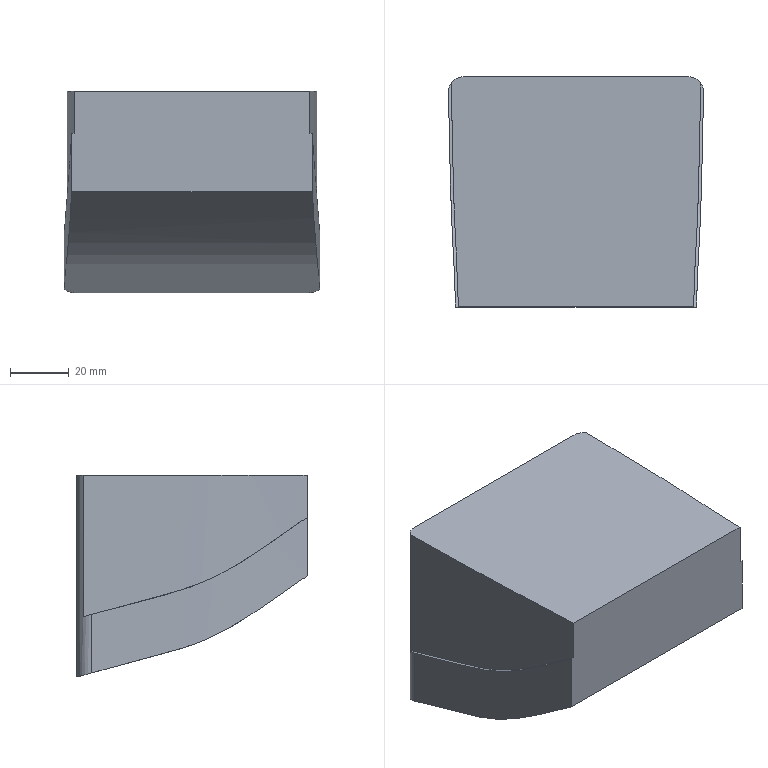Part | NX | features solid 2 | 1 solid | 12 faces | box 87.088 x 78.574 x 68.942 mm | volume 366732 mm3 | spline 7 | plane 3 | cylinder 2 | commonest cylinder face diameters 10 x2
STEP:
#1=CARTESIAN_POINT('',(38.544,100.,30.));
#2=VERTEX_POINT('',#1);
#3=CARTESIAN_POINT('',(-38.544,100.,30.));
#4=VERTEX_POINT('',#3);
#5=CARTESIAN_POINT('',(35.,100.,30.));
#6=DIRECTION('',(1.,0.,0.));
#7=VECTOR('',#6,1000.);
#8=LINE('',#5,#7);
#9=EDGE_CURVE('',#2,#4,#8,.F.);
#10=ORIENTED_EDGE('',*,*,#9,.F.);
#11=CARTESIAN_POINT('',(38.544,100.,-38.942));
#12=VERTEX_POINT('',#11);
#13=CARTESIAN_POINT('',(38.544,100.,-38.942));
#14=DIRECTION('',(0.,0.,1.));
#15=VECTOR('',#14,1000.);
#16=LINE('',#13,#15);
#17=EDGE_CURVE('',#2,#12,#16,.F.);
#18=ORIENTED_EDGE('',*,*,#17,.T.);
#19=CARTESIAN_POINT('',(-38.544,100.,-38.942));
#20=VERTEX_POINT('',#19);
#21=CARTESIAN_POINT('',(0.,100.,-38.942));
#22=DIRECTION('',(1.,0.,0.));
#23=VECTOR('',#22,1000.);
#24=LINE('',#21,#23);
#25=EDGE_CURVE('',#12,#20,#24,.F.);
#26=ORIENTED_EDGE('',*,*,#25,.T.);
#27=CARTESIAN_POINT('',(-38.544,100.,-18.962));
#28=DIRECTION('',(0.,0.,1.));
#29=VECTOR('',#28,1000.);
#30=LINE('',#27,#29);
#31=EDGE_CURVE('',#20,#4,#30,.T.);
#32=ORIENTED_EDGE('',*,*,#31,.T.);
#33=EDGE_LOOP('',(#10,#18,#26,#32));
#34=FACE_BOUND('',#33,.T.);
#35=CARTESIAN_POINT('',(40.,100.,-30.));
#36=DIRECTION('',(0.,1.,0.));
#37=DIRECTION('',(0.,0.,-1.));
#38=AXIS2_PLACEMENT_3D('',#35,#36,#37);
#39=PLANE('',#38);
#40=ADVANCED_FACE('',(#34),#39,.T.);
#41=CARTESIAN_POINT('',(40.161,21.431,15.579));
#42=VERTEX_POINT('',#41);
#43=CARTESIAN_POINT('',(41.123,21.431,15.562));
#44=VERTEX_POINT('',#43);
#45=CARTESIAN_POINT('',(40.161,21.431,15.568));
#46=CARTESIAN_POINT('',(40.482,21.431,15.566));
#47=CARTESIAN_POINT('',(40.802,21.431,15.564));
#48=CARTESIAN_POINT('',(41.123,21.431,15.562));
#49=B_SPLINE_CURVE_WITH_KNOTS('',3,(#45,#46,#47,#48),.UNSPECIFIED.,.F.,.F.,(4,4),(0.003161,0.004123),.UNSPECIFIED.);
#50=EDGE_CURVE('',#42,#44,#49,.T.);
#51=ORIENTED_EDGE('',*,*,#50,.F.);
#52=CARTESIAN_POINT('',(40.161,21.431,30.));
#53=VERTEX_POINT('',#52);
#54=CARTESIAN_POINT('',(40.161,21.431,30.));
#55=DIRECTION('',(0.,0.,1.));
#56=VECTOR('',#55,1000.);
#57=LINE('',#54,#56);
#58=EDGE_CURVE('',#53,#42,#57,.F.);
#59=ORIENTED_EDGE('',*,*,#58,.F.);
#60=CARTESIAN_POINT('',(-40.161,21.431,30.));
#61=VERTEX_POINT('',#60);
#62=CARTESIAN_POINT('',(-41.447,21.431,30.));
#63=DIRECTION('',(-1.,0.,0.));
#64=VECTOR('',#63,1000.);
#65=LINE('',#62,#64);
#66=EDGE_CURVE('',#61,#53,#65,.F.);
#67=ORIENTED_EDGE('',*,*,#66,.F.);
#68=CARTESIAN_POINT('',(-40.161,21.431,15.568));
#69=VERTEX_POINT('',#68);
#70=CARTESIAN_POINT('',(-40.161,21.431,21.029));
#71=DIRECTION('',(0.,0.,1.));
#72=VECTOR('',#71,1000.);
#73=LINE('',#70,#72);
#74=EDGE_CURVE('',#69,#61,#73,.T.);
#75=ORIENTED_EDGE('',*,*,#74,.F.);
#76=CARTESIAN_POINT('',(-41.123,21.431,15.562));
#77=VERTEX_POINT('',#76);
#78=CARTESIAN_POINT('',(-40.161,21.431,15.568));
#79=CARTESIAN_POINT('',(-40.482,21.431,15.566));
#80=CARTESIAN_POINT('',(-40.803,21.431,15.564));
#81=CARTESIAN_POINT('',(-41.123,21.431,15.562));
#82=B_SPLINE_CURVE_WITH_KNOTS('',3,(#78,#79,#80,#81),.UNSPECIFIED.,.F.,.F.,(4,4),(0.003161,0.004123),.UNSPECIFIED.);
#83=EDGE_CURVE('',#77,#69,#82,.F.);
#84=ORIENTED_EDGE('',*,*,#83,.F.);
#85=CARTESIAN_POINT('',(-41.123,21.431,-4.468));
#86=VERTEX_POINT('',#85);
#87=CARTESIAN_POINT('',(-41.123,21.431,2.04));
#88=DIRECTION('',(0.,0.,-1.));
#89=VECTOR('',#88,1000.);
#90=LINE('',#87,#89);
#91=EDGE_CURVE('',#77,#86,#90,.T.);
#92=ORIENTED_EDGE('',*,*,#91,.T.);
#93=CARTESIAN_POINT('',(41.123,21.431,-4.468));
#94=VERTEX_POINT('',#93);
#95=CARTESIAN_POINT('',(0.,21.431,-4.468));
#96=DIRECTION('',(1.,0.,0.));
#97=VECTOR('',#96,1000.);
#98=LINE('',#95,#97);
#99=EDGE_CURVE('',#86,#94,#98,.T.);
#100=ORIENTED_EDGE('',*,*,#99,.T.);
#101=CARTESIAN_POINT('',(41.123,21.431,2.04));
#102=DIRECTION('',(0.,0.,-1.));
#103=VECTOR('',#102,1000.);
#104=LINE('',#101,#103);
#105=EDGE_CURVE('',#44,#94,#104,.T.);
#106=ORIENTED_EDGE('',*,*,#105,.F.);
#107=EDGE_LOOP('',(#51,#59,#67,#75,#84,#92,#100,#106));
#108=FACE_BOUND('',#107,.T.);
#109=CARTESIAN_POINT('',(-41.447,21.431,488.558));
#110=DIRECTION('',(0.,1.,0.));
#111=DIRECTION('',(0.,0.,1.));
#112=AXIS2_PLACEMENT_3D('',#109,#110,#111);
#113=PLANE('',#112);
#114=ADVANCED_FACE('',(#108),#113,.F.);
#115=CARTESIAN_POINT('',(-42.61,97.91,-18.386));
#116=VERTEX_POINT('',#115);
#117=CARTESIAN_POINT('',(-42.61,97.91,-18.386));
#118=CARTESIAN_POINT('',(-42.46,91.108,-16.529));
#119=CARTESIAN_POINT('',(-42.246,80.889,-13.829));
#120=CARTESIAN_POINT('',(-41.958,67.243,-10.237));
#121=CARTESIAN_POINT('',(-41.684,57.189,-6.958));
#122=CARTESIAN_POINT('',(-41.307,47.723,-2.238));
#123=CARTESIAN_POINT('',(-40.788,38.826,3.473));
#124=CARTESIAN_POINT('',(-40.354,30.105,9.464));
#125=CARTESIAN_POINT('',(-40.233,24.323,13.537));
#126=CARTESIAN_POINT('',(-40.161,21.431,15.568));
#127=B_SPLINE_CURVE_WITH_KNOTS('',3,(#117,#118,#119,#120,#121,#122,#123,#124,#125,#126),.UNSPECIFIED.,.F.,.F.,(4,1,1,1,1,1,1,4),(0.776,0.8364,0.8666,0.8968,0.9269,0.9571,0.9873,1.017),.UNSPECIFIED.);
#128=EDGE_CURVE('',#69,#116,#127,.F.);
#129=ORIENTED_EDGE('',*,*,#128,.T.);
#130=CARTESIAN_POINT('',(-43.543,94.893,-17.57));
#131=VERTEX_POINT('',#130);
#132=CARTESIAN_POINT('',(-42.61,97.91,-18.386));
#133=CARTESIAN_POINT('',(-43.244,97.025,-18.148));
#134=CARTESIAN_POINT('',(-43.566,95.968,-17.862));
#135=CARTESIAN_POINT('',(-43.543,94.893,-17.57));
#136=B_SPLINE_CURVE_WITH_KNOTS('',3,(#132,#133,#134,#135),.UNSPECIFIED.,.F.,.F.,(4,4),(0.,0.003307),.UNSPECIFIED.);
#137=EDGE_CURVE('',#116,#131,#136,.T.);
#138=ORIENTED_EDGE('',*,*,#137,.T.);
#139=CARTESIAN_POINT('',(-43.543,94.893,-17.57));
#140=CARTESIAN_POINT('',(-43.403,88.337,-15.791));
#141=CARTESIAN_POINT('',(-43.13,75.203,-12.367));
#142=CARTESIAN_POINT('',(-42.757,58.761,-7.923));
#143=CARTESIAN_POINT('',(-42.26,46.679,-1.63));
#144=CARTESIAN_POINT('',(-41.744,38.142,3.901));
#145=CARTESIAN_POINT('',(-41.371,29.755,9.685));
#146=CARTESIAN_POINT('',(-41.213,24.207,13.606));
#147=CARTESIAN_POINT('',(-41.123,21.431,15.562));
#148=B_SPLINE_CURVE_WITH_KNOTS('',3,(#139,#140,#141,#142,#143,#144,#145,#146,#147),.UNSPECIFIED.,.F.,.F.,(4,1,1,1,1,1,4),(0.2199,0.2402,0.2604,0.2705,0.2806,0.2908,0.3009),.UNSPECIFIED.);
#149=EDGE_CURVE('',#131,#77,#148,.T.);
#150=ORIENTED_EDGE('',*,*,#149,.T.);
#151=ORIENTED_EDGE('',*,*,#83,.T.);
#152=EDGE_LOOP('',(#129,#138,#150,#151));
#153=FACE_BOUND('',#152,.T.);
#154=CARTESIAN_POINT('',(-40.151,21.014,15.861));
#155=CARTESIAN_POINT('',(-40.196,22.828,14.587));
#156=CARTESIAN_POINT('',(-40.241,24.642,13.313));
#157=CARTESIAN_POINT('',(-40.286,26.455,12.04));
#158=CARTESIAN_POINT('',(-40.36,29.45,9.936));
#159=CARTESIAN_POINT('',(-40.476,32.454,7.851));
#160=CARTESIAN_POINT('',(-40.774,38.493,3.743));
#161=CARTESIAN_POINT('',(-40.955,41.527,1.719));
#162=CARTESIAN_POINT('',(-41.288,47.744,-2.094));
#163=CARTESIAN_POINT('',(-41.436,50.935,-3.872));
#164=CARTESIAN_POINT('',(-41.683,57.549,-6.923));
#165=CARTESIAN_POINT('',(-41.786,60.972,-8.184));
#166=CARTESIAN_POINT('',(-41.968,67.929,-10.377));
#167=CARTESIAN_POINT('',(-42.046,71.455,-11.333));
#168=CARTESIAN_POINT('',(-42.196,78.512,-13.21));
#169=CARTESIAN_POINT('',(-42.269,82.045,-14.129));
#170=CARTESIAN_POINT('',(-42.418,89.101,-15.999));
#171=CARTESIAN_POINT('',(-42.494,92.625,-16.947));
#172=CARTESIAN_POINT('',(-42.588,96.898,-18.11));
#173=CARTESIAN_POINT('',(-42.604,97.649,-18.315));
#174=CARTESIAN_POINT('',(-42.621,98.4,-18.52));
#175=CARTESIAN_POINT('',(-41.192,21.005,15.861));
#176=CARTESIAN_POINT('',(-41.237,22.813,14.587));
#177=CARTESIAN_POINT('',(-41.281,24.621,13.313));
#178=CARTESIAN_POINT('',(-41.326,26.43,12.04));
#179=CARTESIAN_POINT('',(-41.4,29.416,9.936));
#180=CARTESIAN_POINT('',(-41.516,32.409,7.851));
#181=CARTESIAN_POINT('',(-41.814,38.435,3.743));
#182=CARTESIAN_POINT('',(-41.994,41.468,1.719));
#183=CARTESIAN_POINT('',(-42.327,47.692,-2.094));
#184=CARTESIAN_POINT('',(-42.476,50.891,-3.872));
#185=CARTESIAN_POINT('',(-42.724,57.516,-6.923));
#186=CARTESIAN_POINT('',(-42.827,60.942,-8.184));
#187=CARTESIAN_POINT('',(-43.009,67.905,-10.377));
#188=CARTESIAN_POINT('',(-43.087,71.433,-11.333));
#189=CARTESIAN_POINT('',(-43.237,78.491,-13.21));
#190=CARTESIAN_POINT('',(-43.309,82.024,-14.129));
#191=CARTESIAN_POINT('',(-43.458,89.079,-15.999));
#192=CARTESIAN_POINT('',(-43.535,92.603,-16.947));
#193=CARTESIAN_POINT('',(-43.628,96.876,-18.11));
#194=CARTESIAN_POINT('',(-43.645,97.626,-18.315));
#195=CARTESIAN_POINT('',(-43.661,98.377,-18.52));
#196=B_SPLINE_SURFACE_WITH_KNOTS('',1,3,((#154,#155,#156,#157,#158,#159,#160,#161,#162,#163,#164,#165,#166,#167,#168,#169,#170,#171,#172,#173,#174),(#175,#176,#177,#178,#179,#180,#181,#182,#183,#184,#185,#186,#187,#188,#189,#190,#191,#192,#193,#194,#195)),.RULED_SURF.,.F.,.F.,.F.,(2,2),(4,3,2,2,2,2,2,2,2,4),(0.,0.3469),(-0.01892,0.,0.03125,0.0625,0.09375,0.125,0.1562,0.1875,0.2188,0.2254),.UNSPECIFIED.);
#197=ADVANCED_FACE('',(#153),#196,.F.);
#198=CARTESIAN_POINT('',(-42.61,97.911,30.));
#199=VERTEX_POINT('',#198);
#200=CARTESIAN_POINT('',(-42.61,97.911,30.));
#201=CARTESIAN_POINT('',(-42.47,91.536,30.));
#202=CARTESIAN_POINT('',(-42.2,78.785,30.));
#203=CARTESIAN_POINT('',(-41.869,62.848,30.));
#204=CARTESIAN_POINT('',(-41.423,50.102,30.));
#205=CARTESIAN_POINT('',(-40.895,40.547,30.));
#206=CARTESIAN_POINT('',(-40.375,30.993,30.));
#207=CARTESIAN_POINT('',(-40.24,24.618,30.));
#208=CARTESIAN_POINT('',(-40.161,21.431,30.));
#209=B_SPLINE_CURVE_WITH_KNOTS('',3,(#200,#201,#202,#203,#204,#205,#206,#207,#208),.UNSPECIFIED.,.F.,.F.,(4,1,1,1,1,1,4),(0.2691,0.2881,0.3071,0.3166,0.3261,0.3356,0.3451),.UNSPECIFIED.);
#210=EDGE_CURVE('',#199,#61,#209,.T.);
#211=ORIENTED_EDGE('',*,*,#210,.F.);
#212=CARTESIAN_POINT('',(-42.61,97.911,30.));
#213=DIRECTION('',(0.,0.,1.));
#214=VECTOR('',#213,1000.);
#215=LINE('',#212,#214);
#216=EDGE_CURVE('',#199,#116,#215,.F.);
#217=ORIENTED_EDGE('',*,*,#216,.T.);
#218=ORIENTED_EDGE('',*,*,#128,.F.);
#219=ORIENTED_EDGE('',*,*,#74,.T.);
#220=EDGE_LOOP('',(#211,#217,#218,#219));
#221=FACE_BOUND('',#220,.T.);
#222=CARTESIAN_POINT('',(-40.161,21.431,15.278));
#223=CARTESIAN_POINT('',(-40.161,21.431,64.255));
#224=CARTESIAN_POINT('',(-40.233,24.333,13.234));
#225=CARTESIAN_POINT('',(-40.233,24.333,62.211));
#226=CARTESIAN_POINT('',(-40.354,30.142,9.137));
#227=CARTESIAN_POINT('',(-40.354,30.142,58.113));
#228=CARTESIAN_POINT('',(-40.794,38.922,3.11));
#229=CARTESIAN_POINT('',(-40.794,38.922,52.087));
#230=CARTESIAN_POINT('',(-41.316,47.874,-2.632));
#231=CARTESIAN_POINT('',(-41.316,47.874,46.344));
#232=CARTESIAN_POINT('',(-41.691,57.414,-7.357));
#233=CARTESIAN_POINT('',(-41.691,57.414,41.62));
#234=CARTESIAN_POINT('',(-41.965,67.544,-10.619));
#235=CARTESIAN_POINT('',(-41.965,67.544,38.358));
#236=CARTESIAN_POINT('',(-42.253,81.274,-14.227));
#237=CARTESIAN_POINT('',(-42.253,81.274,34.749));
#238=CARTESIAN_POINT('',(-42.47,91.555,-16.955));
#239=CARTESIAN_POINT('',(-42.47,91.555,32.022));
#240=CARTESIAN_POINT('',(-42.621,98.401,-18.82));
#241=CARTESIAN_POINT('',(-42.621,98.401,30.157));
#242=B_SPLINE_SURFACE_WITH_KNOTS('',3,1,((#222,#223),(#224,#225),(#226,#227),(#228,#229),(#230,#231),(#232,#233),(#234,#235),(#236,#237),(#238,#239),(#240,#241)),.SURF_OF_LINEAR_EXTRUSION.,.F.,.F.,.F.,(4,1,1,1,1,1,1,4),(2,2),(-0.01753,0.01284,0.04321,0.07358,0.1039,0.1343,0.1647,0.2254),(0.,1.),.UNSPECIFIED.);
#243=ADVANCED_FACE('',(#221),#242,.F.);
#244=ORIENTED_EDGE('',*,*,#25,.F.);
#245=CARTESIAN_POINT('',(43.543,94.893,-37.563));
#246=VERTEX_POINT('',#245);
#247=CARTESIAN_POINT('',(38.544,100.,-38.942));
#248=CARTESIAN_POINT('',(39.908,100.,-38.942));
#249=CARTESIAN_POINT('',(42.556,98.829,-38.625));
#250=CARTESIAN_POINT('',(43.571,96.208,-37.917));
#251=CARTESIAN_POINT('',(43.543,94.893,-37.563));
#252=B_SPLINE_CURVE_WITH_KNOTS('',3,(#247,#248,#249,#250,#251),.UNSPECIFIED.,.F.,.F.,(4,1,4),(0.,0.004031,0.008063),.UNSPECIFIED.);
#253=EDGE_CURVE('',#12,#246,#252,.T.);
#254=ORIENTED_EDGE('',*,*,#253,.T.);
#255=CARTESIAN_POINT('',(43.543,94.893,-37.563));
#256=CARTESIAN_POINT('',(43.402,88.317,-35.793));
#257=CARTESIAN_POINT('',(43.19,78.442,-33.17));
#258=CARTESIAN_POINT('',(42.917,65.276,-29.698));
#259=CARTESIAN_POINT('',(42.626,55.633,-26.315));
#260=CARTESIAN_POINT('',(42.255,46.568,-21.554));
#261=CARTESIAN_POINT('',(41.74,38.077,-16.056));
#262=CARTESIAN_POINT('',(41.371,29.739,-10.283));
#263=CARTESIAN_POINT('',(41.213,24.202,-6.404));
#264=CARTESIAN_POINT('',(41.123,21.431,-4.468));
#265=B_SPLINE_CURVE_WITH_KNOTS('',3,(#255,#256,#257,#258,#259,#260,#261,#262,#263,#264),.UNSPECIFIED.,.F.,.F.,(4,1,1,1,1,1,1,4),(0.1295,0.1497,0.1598,0.1699,0.18,0.1901,0.2002,0.2103),.UNSPECIFIED.);
#266=EDGE_CURVE('',#246,#94,#265,.T.);
#267=ORIENTED_EDGE('',*,*,#266,.T.);
#268=ORIENTED_EDGE('',*,*,#99,.F.);
#269=CARTESIAN_POINT('',(-43.543,94.893,-37.563));
#270=VERTEX_POINT('',#269);
#271=CARTESIAN_POINT('',(-43.543,94.893,-37.563));
#272=CARTESIAN_POINT('',(-43.403,88.345,-35.801));
#273=CARTESIAN_POINT('',(-43.192,78.511,-33.187));
#274=CARTESIAN_POINT('',(-42.92,65.404,-29.733));
#275=CARTESIAN_POINT('',(-42.631,55.762,-26.372));
#276=CARTESIAN_POINT('',(-42.259,46.65,-21.605));
#277=CARTESIAN_POINT('',(-41.743,38.132,-16.094));
#278=CARTESIAN_POINT('',(-41.371,29.766,-10.302));
#279=CARTESIAN_POINT('',(-41.213,24.211,-6.41));
#280=CARTESIAN_POINT('',(-41.123,21.431,-4.468));
#281=B_SPLINE_CURVE_WITH_KNOTS('',3,(#271,#272,#273,#274,#275,#276,#277,#278,#279,#280),.UNSPECIFIED.,.F.,.F.,(4,1,1,1,1,1,1,4),(0.01923,0.03957,0.04975,0.05992,0.07009,0.08026,0.09044,0.1006),.UNSPECIFIED.);
#282=EDGE_CURVE('',#270,#86,#281,.T.);
#283=ORIENTED_EDGE('',*,*,#282,.F.);
#284=CARTESIAN_POINT('',(-43.543,94.893,-37.563));
#285=CARTESIAN_POINT('',(-43.571,96.209,-37.917));
#286=CARTESIAN_POINT('',(-42.56,98.824,-38.624));
#287=CARTESIAN_POINT('',(-39.908,100.,-38.942));
#288=CARTESIAN_POINT('',(-38.544,100.,-38.942));
#289=B_SPLINE_CURVE_WITH_KNOTS('',3,(#284,#285,#286,#287,#288),.UNSPECIFIED.,.F.,.F.,(4,1,4),(0.,0.004031,0.008062),.UNSPECIFIED.);
#290=EDGE_CURVE('',#270,#20,#289,.T.);
#291=ORIENTED_EDGE('',*,*,#290,.T.);
#292=EDGE_LOOP('',(#244,#254,#267,#268,#283,#291));
#293=FACE_BOUND('',#292,.T.);
#294=CARTESIAN_POINT('',(-44.308,100.,-38.942));
#295=CARTESIAN_POINT('',(43.975,100.,-38.942));
#296=CARTESIAN_POINT('',(-44.155,93.019,-37.054));
#297=CARTESIAN_POINT('',(44.127,93.019,-37.054));
#298=CARTESIAN_POINT('',(-43.938,82.545,-34.236));
#299=CARTESIAN_POINT('',(44.345,82.545,-34.236));
#300=CARTESIAN_POINT('',(-43.644,68.55,-30.599));
#301=CARTESIAN_POINT('',(44.638,68.55,-30.599));
#302=CARTESIAN_POINT('',(-43.378,58.17,-27.391));
#303=CARTESIAN_POINT('',(44.905,58.17,-27.391));
#304=CARTESIAN_POINT('',(-42.99,48.384,-22.659));
#305=CARTESIAN_POINT('',(45.293,48.384,-22.659));
#306=CARTESIAN_POINT('',(-42.474,39.233,-16.842));
#307=CARTESIAN_POINT('',(45.808,39.233,-16.842));
#308=CARTESIAN_POINT('',(-42.047,30.309,-10.687));
#309=CARTESIAN_POINT('',(46.236,30.309,-10.687));
#310=CARTESIAN_POINT('',(-41.782,24.393,-6.537));
#311=CARTESIAN_POINT('',(46.501,24.393,-6.537));
#312=CARTESIAN_POINT('',(-41.647,21.431,-4.468));
#313=CARTESIAN_POINT('',(46.636,21.431,-4.468));
#314=B_SPLINE_SURFACE_WITH_KNOTS('',3,1,((#294,#295),(#296,#297),(#298,#299),(#300,#301),(#302,#303),(#304,#305),(#306,#307),(#308,#309),(#310,#311),(#312,#313)),.SURF_OF_LINEAR_EXTRUSION.,.F.,.F.,.F.,(4,1,1,1,1,1,1,4),(2,2),(0.7835,0.8465,0.878,0.9095,0.941,0.9725,1.004,1.035),(0.,1.),.UNSPECIFIED.);
#315=ADVANCED_FACE('',(#293),#314,.F.);
#316=ORIENTED_EDGE('',*,*,#149,.F.);
#317=CARTESIAN_POINT('',(-43.543,94.893,-17.57));
#318=DIRECTION('',(0.,0.,-1.));
#319=VECTOR('',#318,1000.);
#320=LINE('',#317,#319);
#321=EDGE_CURVE('',#131,#270,#320,.T.);
#322=ORIENTED_EDGE('',*,*,#321,.T.);
#323=ORIENTED_EDGE('',*,*,#282,.T.);
#324=ORIENTED_EDGE('',*,*,#91,.F.);
#325=EDGE_LOOP('',(#316,#322,#323,#324));
#326=FACE_BOUND('',#325,.T.);
#327=CARTESIAN_POINT('',(-43.543,94.893,-17.312));
#328=CARTESIAN_POINT('',(-43.543,94.893,-37.761));
#329=CARTESIAN_POINT('',(-43.403,88.338,-15.559));
#330=CARTESIAN_POINT('',(-43.403,88.338,-36.009));
#331=CARTESIAN_POINT('',(-43.192,78.51,-12.929));
#332=CARTESIAN_POINT('',(-43.192,78.51,-33.378));
#333=CARTESIAN_POINT('',(-42.919,65.37,-9.505));
#334=CARTESIAN_POINT('',(-42.919,65.37,-29.955));
#335=CARTESIAN_POINT('',(-42.632,55.789,-6.049));
#336=CARTESIAN_POINT('',(-42.632,55.789,-26.499));
#337=CARTESIAN_POINT('',(-42.26,46.675,-1.476));
#338=CARTESIAN_POINT('',(-42.26,46.675,-21.926));
#339=CARTESIAN_POINT('',(-41.749,38.218,4.18));
#340=CARTESIAN_POINT('',(-41.749,38.218,-16.27));
#341=CARTESIAN_POINT('',(-41.372,29.817,9.913));
#342=CARTESIAN_POINT('',(-41.372,29.817,-10.537));
#343=CARTESIAN_POINT('',(-41.214,24.227,13.762));
#344=CARTESIAN_POINT('',(-41.214,24.227,-6.688));
#345=CARTESIAN_POINT('',(-41.123,21.431,15.683));
#346=CARTESIAN_POINT('',(-41.123,21.431,-4.767));
#347=B_SPLINE_SURFACE_WITH_KNOTS('',3,1,((#327,#328),(#329,#330),(#331,#332),(#333,#334),(#335,#336),(#337,#338),(#339,#340),(#341,#342),(#343,#344),(#345,#346)),.SURF_OF_LINEAR_EXTRUSION.,.F.,.F.,.F.,(4,1,1,1,1,1,1,4),(2,2),(0.7971,0.8567,0.8865,0.9163,0.9461,0.9759,1.006,1.036),(0.,1.),.UNSPECIFIED.);
#348=ADVANCED_FACE('',(#326),#347,.F.);
#349=CARTESIAN_POINT('',(43.543,94.893,-17.57));
#350=VERTEX_POINT('',#349);
#351=CARTESIAN_POINT('',(41.123,21.431,15.562));
#352=CARTESIAN_POINT('',(41.213,24.208,13.605));
#353=CARTESIAN_POINT('',(41.371,29.757,9.683));
#354=CARTESIAN_POINT('',(41.744,38.144,3.899));
#355=CARTESIAN_POINT('',(42.26,46.687,-1.635));
#356=CARTESIAN_POINT('',(42.758,58.766,-7.924));
#357=CARTESIAN_POINT('',(43.131,75.218,-12.371));
#358=CARTESIAN_POINT('',(43.403,88.34,-15.792));
#359=CARTESIAN_POINT('',(43.543,94.893,-17.57));
#360=B_SPLINE_CURVE_WITH_KNOTS('',3,(#351,#352,#353,#354,#355,#356,#357,#358,#359),.UNSPECIFIED.,.F.,.F.,(4,1,1,1,1,1,4),(-0.006118,0.004077,0.01427,0.02447,0.03466,0.05505,0.07544),.UNSPECIFIED.);
#361=EDGE_CURVE('',#44,#350,#360,.T.);
#362=ORIENTED_EDGE('',*,*,#361,.T.);
#363=CARTESIAN_POINT('',(42.61,97.91,-18.386));
#364=VERTEX_POINT('',#363);
#365=CARTESIAN_POINT('',(43.543,94.893,-17.57));
#366=CARTESIAN_POINT('',(43.566,95.968,-17.862));
#367=CARTESIAN_POINT('',(43.244,97.025,-18.148));
#368=CARTESIAN_POINT('',(42.61,97.91,-18.386));
#369=B_SPLINE_CURVE_WITH_KNOTS('',3,(#365,#366,#367,#368),.UNSPECIFIED.,.F.,.F.,(4,4),(0.,0.003308),.UNSPECIFIED.);
#370=EDGE_CURVE('',#350,#364,#369,.T.);
#371=ORIENTED_EDGE('',*,*,#370,.T.);
#372=CARTESIAN_POINT('',(42.61,97.91,-18.386));
#373=CARTESIAN_POINT('',(42.46,91.107,-16.529));
#374=CARTESIAN_POINT('',(42.246,80.887,-13.828));
#375=CARTESIAN_POINT('',(41.958,67.241,-10.236));
#376=CARTESIAN_POINT('',(41.684,57.186,-6.957));
#377=CARTESIAN_POINT('',(41.307,47.719,-2.236));
#378=CARTESIAN_POINT('',(40.788,38.823,3.476));
#379=CARTESIAN_POINT('',(40.354,30.101,9.467));
#380=CARTESIAN_POINT('',(40.233,24.318,13.54));
#381=CARTESIAN_POINT('',(40.161,21.426,15.572));
#382=B_SPLINE_CURVE_WITH_KNOTS('',3,(#372,#373,#374,#375,#376,#377,#378,#379,#380,#381),.UNSPECIFIED.,.F.,.F.,(4,1,1,1,1,1,1,4),(0.776,0.8364,0.8666,0.8968,0.9269,0.9571,0.9873,1.017),.UNSPECIFIED.);
#383=EDGE_CURVE('',#42,#364,#382,.F.);
#384=ORIENTED_EDGE('',*,*,#383,.F.);
#385=ORIENTED_EDGE('',*,*,#50,.T.);
#386=EDGE_LOOP('',(#362,#371,#384,#385));
#387=FACE_BOUND('',#386,.T.);
#388=CARTESIAN_POINT('',(40.145,21.009,15.864));
#389=CARTESIAN_POINT('',(40.19,22.825,14.59));
#390=CARTESIAN_POINT('',(40.235,24.64,13.315));
#391=CARTESIAN_POINT('',(40.279,26.455,12.04));
#392=CARTESIAN_POINT('',(40.354,29.451,9.936));
#393=CARTESIAN_POINT('',(40.47,32.454,7.851));
#394=CARTESIAN_POINT('',(40.768,38.494,3.743));
#395=CARTESIAN_POINT('',(40.949,41.528,1.719));
#396=CARTESIAN_POINT('',(41.281,47.744,-2.094));
#397=CARTESIAN_POINT('',(41.429,50.935,-3.872));
#398=CARTESIAN_POINT('',(41.677,57.549,-6.923));
#399=CARTESIAN_POINT('',(41.78,60.972,-8.184));
#400=CARTESIAN_POINT('',(41.962,67.929,-10.377));
#401=CARTESIAN_POINT('',(42.04,71.456,-11.333));
#402=CARTESIAN_POINT('',(42.19,78.512,-13.21));
#403=CARTESIAN_POINT('',(42.263,82.046,-14.129));
#404=CARTESIAN_POINT('',(42.412,89.102,-15.999));
#405=CARTESIAN_POINT('',(42.488,92.625,-16.947));
#406=CARTESIAN_POINT('',(42.581,96.899,-18.11));
#407=CARTESIAN_POINT('',(42.598,97.649,-18.315));
#408=CARTESIAN_POINT('',(42.614,98.4,-18.52));
#409=CARTESIAN_POINT('',(40.151,21.009,15.864));
#410=CARTESIAN_POINT('',(40.196,22.824,14.59));
#411=CARTESIAN_POINT('',(40.241,24.64,13.315));
#412=CARTESIAN_POINT('',(40.286,26.455,12.04));
#413=CARTESIAN_POINT('',(40.36,29.45,9.936));
#414=CARTESIAN_POINT('',(40.476,32.454,7.851));
#415=CARTESIAN_POINT('',(40.774,38.493,3.743));
#416=CARTESIAN_POINT('',(40.955,41.527,1.719));
#417=CARTESIAN_POINT('',(41.288,47.744,-2.094));
#418=CARTESIAN_POINT('',(41.436,50.935,-3.872));
#419=CARTESIAN_POINT('',(41.683,57.549,-6.923));
#420=CARTESIAN_POINT('',(41.786,60.972,-8.184));
#421=CARTESIAN_POINT('',(41.968,67.929,-10.377));
#422=CARTESIAN_POINT('',(42.046,71.455,-11.333));
#423=CARTESIAN_POINT('',(42.196,78.512,-13.21));
#424=CARTESIAN_POINT('',(42.269,82.045,-14.129));
#425=CARTESIAN_POINT('',(42.418,89.101,-15.999));
#426=CARTESIAN_POINT('',(42.494,92.625,-16.947));
#427=CARTESIAN_POINT('',(42.588,96.898,-18.11));
#428=CARTESIAN_POINT('',(42.604,97.649,-18.315));
#429=CARTESIAN_POINT('',(42.621,98.4,-18.52));
#430=CARTESIAN_POINT('',(41.17,21.,15.865));
#431=CARTESIAN_POINT('',(41.215,22.81,14.59));
#432=CARTESIAN_POINT('',(41.259,24.62,13.315));
#433=CARTESIAN_POINT('',(41.304,26.43,12.04));
#434=CARTESIAN_POINT('',(41.378,29.416,9.936));
#435=CARTESIAN_POINT('',(41.494,32.41,7.851));
#436=CARTESIAN_POINT('',(41.792,38.436,3.743));
#437=CARTESIAN_POINT('',(41.972,41.469,1.719));
#438=CARTESIAN_POINT('',(42.305,47.693,-2.094));
#439=CARTESIAN_POINT('',(42.454,50.892,-3.872));
#440=CARTESIAN_POINT('',(42.702,57.516,-6.923));
#441=CARTESIAN_POINT('',(42.805,60.942,-8.184));
#442=CARTESIAN_POINT('',(42.987,67.905,-10.377));
#443=CARTESIAN_POINT('',(43.065,71.433,-11.333));
#444=CARTESIAN_POINT('',(43.215,78.491,-13.21));
#445=CARTESIAN_POINT('',(43.287,82.024,-14.129));
#446=CARTESIAN_POINT('',(43.436,89.08,-15.999));
#447=CARTESIAN_POINT('',(43.513,92.603,-16.947));
#448=CARTESIAN_POINT('',(43.606,96.876,-18.11));
#449=CARTESIAN_POINT('',(43.623,97.627,-18.315));
#450=CARTESIAN_POINT('',(43.639,98.378,-18.52));
#451=B_SPLINE_SURFACE_WITH_KNOTS('',1,3,((#388,#389,#390,#391,#392,#393,#394,#395,#396,#397,#398,#399,#400,#401,#402,#403,#404,#405,#406,#407,#408),(#409,#410,#411,#412,#413,#414,#415,#416,#417,#418,#419,#420,#421,#422,#423,#424,#425,#426,#427,#428,#429),(#430,#431,#432,#433,#434,#435,#436,#437,#438,#439,#440,#441,#442,#443,#444,#445,#446,#447,#448,#449,#450)),.RULED_SURF.,.F.,.F.,.F.,(2,1,2),(4,3,2,2,2,2,2,2,2,4),(-0.00205,0.,0.3396),(-0.01894,0.,0.03125,0.0625,0.09375,0.125,0.1562,0.1875,0.2188,0.2254),.UNSPECIFIED.);
#452=ADVANCED_FACE('',(#387),#451,.T.);
#453=ORIENTED_EDGE('',*,*,#383,.T.);
#454=CARTESIAN_POINT('',(42.61,97.911,30.));
#455=VERTEX_POINT('',#454);
#456=CARTESIAN_POINT('',(42.61,97.911,-18.386));
#457=DIRECTION('',(0.,0.,1.));
#458=VECTOR('',#457,1000.);
#459=LINE('',#456,#458);
#460=EDGE_CURVE('',#364,#455,#459,.T.);
#461=ORIENTED_EDGE('',*,*,#460,.T.);
#462=CARTESIAN_POINT('',(40.161,21.431,30.));
#463=CARTESIAN_POINT('',(40.24,24.618,30.));
#464=CARTESIAN_POINT('',(40.375,30.993,30.));
#465=CARTESIAN_POINT('',(40.895,40.548,30.));
#466=CARTESIAN_POINT('',(41.423,50.103,30.));
#467=CARTESIAN_POINT('',(41.869,62.849,30.));
#468=CARTESIAN_POINT('',(42.2,78.786,30.));
#469=CARTESIAN_POINT('',(42.47,91.536,30.));
#470=CARTESIAN_POINT('',(42.61,97.911,30.));
#471=B_SPLINE_CURVE_WITH_KNOTS('',3,(#462,#463,#464,#465,#466,#467,#468,#469,#470),.UNSPECIFIED.,.F.,.F.,(4,1,1,1,1,1,4),(-0.005002,0.004563,0.01413,0.02369,0.03326,0.05239,0.07151),.UNSPECIFIED.);
#472=EDGE_CURVE('',#53,#455,#471,.T.);
#473=ORIENTED_EDGE('',*,*,#472,.F.);
#474=ORIENTED_EDGE('',*,*,#58,.T.);
#475=EDGE_LOOP('',(#453,#461,#473,#474));
#476=FACE_BOUND('',#475,.T.);
#477=CARTESIAN_POINT('',(40.161,21.431,15.288));
#478=CARTESIAN_POINT('',(40.161,21.431,64.255));
#479=CARTESIAN_POINT('',(40.233,24.333,13.244));
#480=CARTESIAN_POINT('',(40.233,24.333,62.21));
#481=CARTESIAN_POINT('',(40.354,30.142,9.147));
#482=CARTESIAN_POINT('',(40.354,30.142,58.113));
#483=CARTESIAN_POINT('',(40.794,38.922,3.12));
#484=CARTESIAN_POINT('',(40.794,38.922,52.087));
#485=CARTESIAN_POINT('',(41.316,47.874,-2.622));
#486=CARTESIAN_POINT('',(41.316,47.874,46.344));
#487=CARTESIAN_POINT('',(41.691,57.414,-7.347));
#488=CARTESIAN_POINT('',(41.691,57.414,41.62));
#489=CARTESIAN_POINT('',(41.965,67.544,-10.609));
#490=CARTESIAN_POINT('',(41.965,67.544,38.358));
#491=CARTESIAN_POINT('',(42.253,81.274,-14.217));
#492=CARTESIAN_POINT('',(42.253,81.274,34.749));
#493=CARTESIAN_POINT('',(42.47,91.555,-16.945));
#494=CARTESIAN_POINT('',(42.47,91.555,32.022));
#495=CARTESIAN_POINT('',(42.621,98.401,-18.81));
#496=CARTESIAN_POINT('',(42.621,98.401,30.157));
#497=B_SPLINE_SURFACE_WITH_KNOTS('',3,1,((#477,#478),(#479,#480),(#481,#482),(#483,#484),(#485,#486),(#487,#488),(#489,#490),(#491,#492),(#493,#494),(#495,#496)),.SURF_OF_LINEAR_EXTRUSION.,.F.,.F.,.F.,(4,1,1,1,1,1,1,4),(2,2),(-0.01753,0.01284,0.04321,0.07358,0.1039,0.1343,0.1647,0.2254),(0.,1.),.UNSPECIFIED.);
#498=ADVANCED_FACE('',(#476),#497,.T.);
#499=ORIENTED_EDGE('',*,*,#266,.F.);
#500=CARTESIAN_POINT('',(43.543,94.893,-37.563));
#501=DIRECTION('',(0.,0.,-1.));
#502=VECTOR('',#501,1000.);
#503=LINE('',#500,#502);
#504=EDGE_CURVE('',#246,#350,#503,.F.);
#505=ORIENTED_EDGE('',*,*,#504,.T.);
#506=ORIENTED_EDGE('',*,*,#361,.F.);
#507=ORIENTED_EDGE('',*,*,#105,.T.);
#508=EDGE_LOOP('',(#499,#505,#506,#507));
#509=FACE_BOUND('',#508,.T.);
#510=CARTESIAN_POINT('',(43.543,94.893,-17.312));
#511=CARTESIAN_POINT('',(43.543,94.893,-37.736));
#512=CARTESIAN_POINT('',(43.403,88.338,-15.56));
#513=CARTESIAN_POINT('',(43.403,88.338,-35.984));
#514=CARTESIAN_POINT('',(43.192,78.51,-12.929));
#515=CARTESIAN_POINT('',(43.192,78.51,-33.353));
#516=CARTESIAN_POINT('',(42.919,65.37,-9.505));
#517=CARTESIAN_POINT('',(42.919,65.37,-29.929));
#518=CARTESIAN_POINT('',(42.632,55.789,-6.049));
#519=CARTESIAN_POINT('',(42.632,55.789,-26.474));
#520=CARTESIAN_POINT('',(42.26,46.675,-1.476));
#521=CARTESIAN_POINT('',(42.26,46.675,-21.9));
#522=CARTESIAN_POINT('',(41.749,38.218,4.18));
#523=CARTESIAN_POINT('',(41.749,38.218,-16.245));
#524=CARTESIAN_POINT('',(41.372,29.817,9.913));
#525=CARTESIAN_POINT('',(41.372,29.817,-10.511));
#526=CARTESIAN_POINT('',(41.214,24.227,13.762));
#527=CARTESIAN_POINT('',(41.214,24.227,-6.662));
#528=CARTESIAN_POINT('',(41.123,21.431,15.683));
#529=CARTESIAN_POINT('',(41.123,21.431,-4.741));
#530=B_SPLINE_SURFACE_WITH_KNOTS('',3,1,((#510,#511),(#512,#513),(#514,#515),(#516,#517),(#518,#519),(#520,#521),(#522,#523),(#524,#525),(#526,#527),(#528,#529)),.SURF_OF_LINEAR_EXTRUSION.,.F.,.F.,.F.,(4,1,1,1,1,1,1,4),(2,2),(0.7971,0.8567,0.8865,0.9163,0.9461,0.9759,1.006,1.036),(0.,1.),.UNSPECIFIED.);
#531=ADVANCED_FACE('',(#509),#530,.T.);
#532=ORIENTED_EDGE('',*,*,#472,.T.);
#533=CARTESIAN_POINT('',(38.544,95.,30.));
#534=DIRECTION('',(0.,0.,-1.));
#535=DIRECTION('',(-1.,0.,0.));
#536=AXIS2_PLACEMENT_3D('',#533,#534,#535);
#537=CIRCLE('',#536,5.);
#538=EDGE_CURVE('',#455,#2,#537,.F.);
#539=ORIENTED_EDGE('',*,*,#538,.T.);
#540=ORIENTED_EDGE('',*,*,#9,.T.);
#541=CARTESIAN_POINT('',(-38.544,95.,30.));
#542=DIRECTION('',(0.,0.,-1.));
#543=DIRECTION('',(-1.,0.,0.));
#544=AXIS2_PLACEMENT_3D('',#541,#542,#543);
#545=CIRCLE('',#544,5.);
#546=EDGE_CURVE('',#4,#199,#545,.F.);
#547=ORIENTED_EDGE('',*,*,#546,.T.);
#548=ORIENTED_EDGE('',*,*,#210,.T.);
#549=ORIENTED_EDGE('',*,*,#66,.T.);
#550=EDGE_LOOP('',(#532,#539,#540,#547,#548,#549));
#551=FACE_BOUND('',#550,.T.);
#552=CARTESIAN_POINT('',(35.,380.,30.));
#553=DIRECTION('',(0.,0.,-1.));
#554=DIRECTION('',(-1.,0.,0.));
#555=AXIS2_PLACEMENT_3D('',#552,#553,#554);
#556=PLANE('',#555);
#557=ADVANCED_FACE('',(#551),#556,.F.);
#558=ORIENTED_EDGE('',*,*,#290,.F.);
#559=ORIENTED_EDGE('',*,*,#321,.F.);
#560=ORIENTED_EDGE('',*,*,#137,.F.);
#561=ORIENTED_EDGE('',*,*,#216,.F.);
#562=ORIENTED_EDGE('',*,*,#546,.F.);
#563=ORIENTED_EDGE('',*,*,#31,.F.);
#564=EDGE_LOOP('',(#558,#559,#560,#561,#562,#563));
#565=FACE_BOUND('',#564,.T.);
#566=CARTESIAN_POINT('',(-38.544,95.,-28.952));
#567=DIRECTION('',(0.,0.,-1.));
#568=DIRECTION('',(-1.,0.,0.));
#569=AXIS2_PLACEMENT_3D('',#566,#567,#568);
#570=CYLINDRICAL_SURFACE('',#569,5.);
#571=ADVANCED_FACE('',(#565),#570,.T.);
#572=ORIENTED_EDGE('',*,*,#370,.F.);
#573=ORIENTED_EDGE('',*,*,#504,.F.);
#574=ORIENTED_EDGE('',*,*,#253,.F.);
#575=ORIENTED_EDGE('',*,*,#17,.F.);
#576=ORIENTED_EDGE('',*,*,#538,.F.);
#577=ORIENTED_EDGE('',*,*,#460,.F.);
#578=EDGE_LOOP('',(#572,#573,#574,#575,#576,#577));
#579=FACE_BOUND('',#578,.T.);
#580=CARTESIAN_POINT('',(38.544,95.,-28.952));
#581=DIRECTION('',(0.,0.,-1.));
#582=DIRECTION('',(-1.,0.,0.));
#583=AXIS2_PLACEMENT_3D('',#580,#581,#582);
#584=CYLINDRICAL_SURFACE('',#583,5.);
#585=ADVANCED_FACE('',(#579),#584,.T.);
#586=CLOSED_SHELL('',(#40,#114,#197,#243,#315,#348,#452,#498,#531,#557,#571,#585));
#587=MANIFOLD_SOLID_BREP('',#586);
#588=(LENGTH_UNIT()NAMED_UNIT(*)SI_UNIT(.MILLI.,.METRE.));
#589=UNCERTAINTY_MEASURE_WITH_UNIT(LENGTH_MEASURE(0.0508),#588,'','');
#590=(NAMED_UNIT(*)PLANE_ANGLE_UNIT()SI_UNIT($,.RADIAN.));
#591=(NAMED_UNIT(*)SI_UNIT($,.STERADIAN.)SOLID_ANGLE_UNIT());
#592=(GEOMETRIC_REPRESENTATION_CONTEXT(3)GLOBAL_UNCERTAINTY_ASSIGNED_CONTEXT((#589))GLOBAL_UNIT_ASSIGNED_CONTEXT((#588,#590,#591))REPRESENTATION_CONTEXT('',''));
#593=ADVANCED_BREP_SHAPE_REPRESENTATION('',(#587),#592);